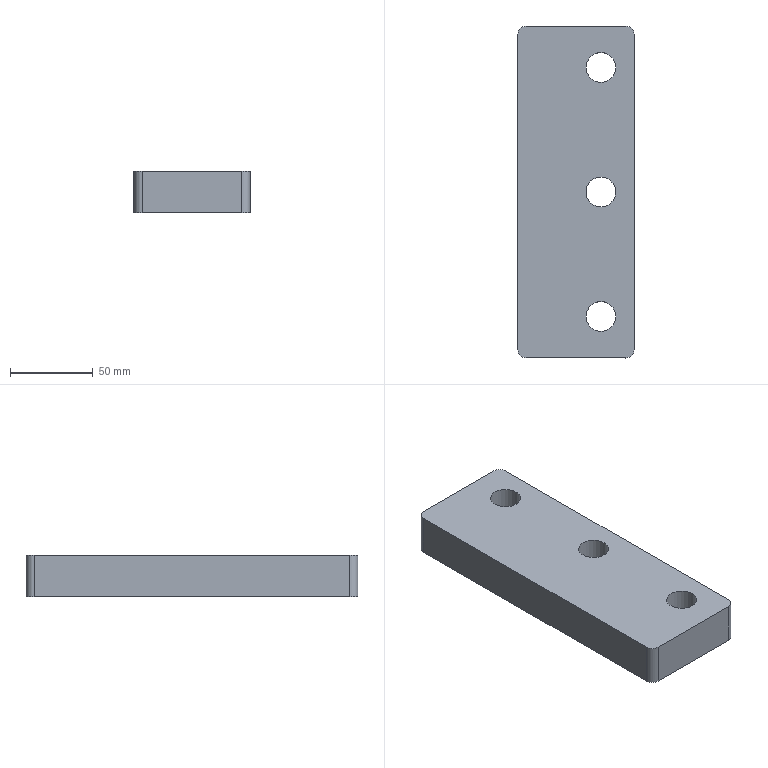Part | NX | features MAIN_BODY 2 | 1 solid | 13 faces | box 70 x 200 x 25 mm | volume 330378 mm3 | cylinder 7 | plane 6 | commonest cylinder face diameters 10 x4 18 x3
STEP:
#1=CARTESIAN_POINT('',(590.,740.,55.));
#2=VERTEX_POINT('',#1);
#3=CARTESIAN_POINT('',(650.,740.,55.));
#4=VERTEX_POINT('',#3);
#5=CARTESIAN_POINT('',(585.,740.,55.));
#6=DIRECTION('',(1.,0.,0.));
#7=VECTOR('',#6,1000.);
#8=LINE('',#5,#7);
#9=EDGE_CURVE('',#2,#4,#8,.T.);
#10=ORIENTED_EDGE('',*,*,#9,.T.);
#11=CARTESIAN_POINT('',(650.,740.,30.));
#12=VERTEX_POINT('',#11);
#13=CARTESIAN_POINT('',(650.,740.,30.));
#14=DIRECTION('',(0.,0.,1.));
#15=VECTOR('',#14,1000.);
#16=LINE('',#13,#15);
#17=EDGE_CURVE('',#12,#4,#16,.T.);
#18=ORIENTED_EDGE('',*,*,#17,.F.);
#19=CARTESIAN_POINT('',(590.,740.,30.));
#20=VERTEX_POINT('',#19);
#21=CARTESIAN_POINT('',(585.,740.,30.));
#22=DIRECTION('',(1.,0.,0.));
#23=VECTOR('',#22,1000.);
#24=LINE('',#21,#23);
#25=EDGE_CURVE('',#20,#12,#24,.T.);
#26=ORIENTED_EDGE('',*,*,#25,.F.);
#27=CARTESIAN_POINT('',(590.,740.,30.));
#28=DIRECTION('',(0.,0.,1.));
#29=VECTOR('',#28,1000.);
#30=LINE('',#27,#29);
#31=EDGE_CURVE('',#2,#20,#30,.F.);
#32=ORIENTED_EDGE('',*,*,#31,.F.);
#33=EDGE_LOOP('',(#10,#18,#26,#32));
#34=FACE_BOUND('',#33,.T.);
#35=CARTESIAN_POINT('',(585.,740.,30.));
#36=DIRECTION('',(0.,1.,0.));
#37=DIRECTION('',(-1.,0.,0.));
#38=AXIS2_PLACEMENT_3D('',#35,#36,#37);
#39=PLANE('',#38);
#40=ADVANCED_FACE('',(#34),#39,.T.);
#41=CARTESIAN_POINT('',(655.,735.,30.));
#42=VERTEX_POINT('',#41);
#43=CARTESIAN_POINT('',(655.,545.,30.));
#44=VERTEX_POINT('',#43);
#45=CARTESIAN_POINT('',(655.,740.,30.));
#46=DIRECTION('',(0.,-1.,0.));
#47=VECTOR('',#46,1000.);
#48=LINE('',#45,#47);
#49=EDGE_CURVE('',#42,#44,#48,.T.);
#50=ORIENTED_EDGE('',*,*,#49,.F.);
#51=CARTESIAN_POINT('',(655.,735.,55.));
#52=VERTEX_POINT('',#51);
#53=CARTESIAN_POINT('',(655.,735.,30.));
#54=DIRECTION('',(0.,0.,1.));
#55=VECTOR('',#54,1000.);
#56=LINE('',#53,#55);
#57=EDGE_CURVE('',#52,#42,#56,.F.);
#58=ORIENTED_EDGE('',*,*,#57,.F.);
#59=CARTESIAN_POINT('',(655.,545.,55.));
#60=VERTEX_POINT('',#59);
#61=CARTESIAN_POINT('',(655.,740.,55.));
#62=DIRECTION('',(0.,-1.,0.));
#63=VECTOR('',#62,1000.);
#64=LINE('',#61,#63);
#65=EDGE_CURVE('',#52,#60,#64,.T.);
#66=ORIENTED_EDGE('',*,*,#65,.T.);
#67=CARTESIAN_POINT('',(655.,545.,30.));
#68=DIRECTION('',(0.,0.,1.));
#69=VECTOR('',#68,1000.);
#70=LINE('',#67,#69);
#71=EDGE_CURVE('',#44,#60,#70,.T.);
#72=ORIENTED_EDGE('',*,*,#71,.F.);
#73=EDGE_LOOP('',(#50,#58,#66,#72));
#74=FACE_BOUND('',#73,.T.);
#75=CARTESIAN_POINT('',(655.,740.,30.));
#76=DIRECTION('',(1.,0.,0.));
#77=DIRECTION('',(0.,1.,0.));
#78=AXIS2_PLACEMENT_3D('',#75,#76,#77);
#79=PLANE('',#78);
#80=ADVANCED_FACE('',(#74),#79,.T.);
#81=CARTESIAN_POINT('',(650.,540.,30.));
#82=VERTEX_POINT('',#81);
#83=CARTESIAN_POINT('',(590.,540.,30.));
#84=VERTEX_POINT('',#83);
#85=CARTESIAN_POINT('',(655.,540.,30.));
#86=DIRECTION('',(-1.,0.,0.));
#87=VECTOR('',#86,1000.);
#88=LINE('',#85,#87);
#89=EDGE_CURVE('',#82,#84,#88,.T.);
#90=ORIENTED_EDGE('',*,*,#89,.F.);
#91=CARTESIAN_POINT('',(650.,540.,55.));
#92=VERTEX_POINT('',#91);
#93=CARTESIAN_POINT('',(650.,540.,30.));
#94=DIRECTION('',(0.,0.,1.));
#95=VECTOR('',#94,1000.);
#96=LINE('',#93,#95);
#97=EDGE_CURVE('',#92,#82,#96,.F.);
#98=ORIENTED_EDGE('',*,*,#97,.F.);
#99=CARTESIAN_POINT('',(590.,540.,55.));
#100=VERTEX_POINT('',#99);
#101=CARTESIAN_POINT('',(655.,540.,55.));
#102=DIRECTION('',(-1.,0.,0.));
#103=VECTOR('',#102,1000.);
#104=LINE('',#101,#103);
#105=EDGE_CURVE('',#92,#100,#104,.T.);
#106=ORIENTED_EDGE('',*,*,#105,.T.);
#107=CARTESIAN_POINT('',(590.,540.,30.));
#108=DIRECTION('',(0.,0.,1.));
#109=VECTOR('',#108,1000.);
#110=LINE('',#107,#109);
#111=EDGE_CURVE('',#84,#100,#110,.T.);
#112=ORIENTED_EDGE('',*,*,#111,.F.);
#113=EDGE_LOOP('',(#90,#98,#106,#112));
#114=FACE_BOUND('',#113,.T.);
#115=CARTESIAN_POINT('',(655.,540.,30.));
#116=DIRECTION('',(0.,-1.,0.));
#117=DIRECTION('',(0.,0.,-1.));
#118=AXIS2_PLACEMENT_3D('',#115,#116,#117);
#119=PLANE('',#118);
#120=ADVANCED_FACE('',(#114),#119,.T.);
#121=CARTESIAN_POINT('',(585.,545.,55.));
#122=VERTEX_POINT('',#121);
#123=CARTESIAN_POINT('',(585.,735.,55.));
#124=VERTEX_POINT('',#123);
#125=CARTESIAN_POINT('',(585.,540.,55.));
#126=DIRECTION('',(0.,1.,0.));
#127=VECTOR('',#126,1000.);
#128=LINE('',#125,#127);
#129=EDGE_CURVE('',#122,#124,#128,.T.);
#130=ORIENTED_EDGE('',*,*,#129,.T.);
#131=CARTESIAN_POINT('',(585.,735.,30.));
#132=VERTEX_POINT('',#131);
#133=CARTESIAN_POINT('',(585.,735.,30.));
#134=DIRECTION('',(0.,0.,1.));
#135=VECTOR('',#134,1000.);
#136=LINE('',#133,#135);
#137=EDGE_CURVE('',#132,#124,#136,.T.);
#138=ORIENTED_EDGE('',*,*,#137,.F.);
#139=CARTESIAN_POINT('',(585.,545.,30.));
#140=VERTEX_POINT('',#139);
#141=CARTESIAN_POINT('',(585.,540.,30.));
#142=DIRECTION('',(0.,1.,0.));
#143=VECTOR('',#142,1000.);
#144=LINE('',#141,#143);
#145=EDGE_CURVE('',#140,#132,#144,.T.);
#146=ORIENTED_EDGE('',*,*,#145,.F.);
#147=CARTESIAN_POINT('',(585.,545.,30.));
#148=DIRECTION('',(0.,0.,1.));
#149=VECTOR('',#148,1000.);
#150=LINE('',#147,#149);
#151=EDGE_CURVE('',#122,#140,#150,.F.);
#152=ORIENTED_EDGE('',*,*,#151,.F.);
#153=EDGE_LOOP('',(#130,#138,#146,#152));
#154=FACE_BOUND('',#153,.T.);
#155=CARTESIAN_POINT('',(585.,540.,30.));
#156=DIRECTION('',(-1.,0.,0.));
#157=DIRECTION('',(0.,0.,-1.));
#158=AXIS2_PLACEMENT_3D('',#155,#156,#157);
#159=PLANE('',#158);
#160=ADVANCED_FACE('',(#154),#159,.T.);
#161=CARTESIAN_POINT('',(635.,556.,30.));
#162=VERTEX_POINT('',#161);
#163=CARTESIAN_POINT('',(635.,565.,30.));
#164=DIRECTION('',(0.,0.,-1.));
#165=DIRECTION('',(0.,-1.,0.));
#166=AXIS2_PLACEMENT_3D('',#163,#164,#165);
#167=CIRCLE('',#166,9.);
#168=EDGE_CURVE('',#162,#162,#167,.T.);
#169=ORIENTED_EDGE('',*,*,#168,.F.);
#170=EDGE_LOOP('',(#169));
#171=FACE_BOUND('',#170,.T.);
#172=CARTESIAN_POINT('',(635.,631.,30.));
#173=VERTEX_POINT('',#172);
#174=CARTESIAN_POINT('',(635.,640.,30.));
#175=DIRECTION('',(0.,0.,-1.));
#176=DIRECTION('',(0.,-1.,0.));
#177=AXIS2_PLACEMENT_3D('',#174,#175,#176);
#178=CIRCLE('',#177,9.);
#179=EDGE_CURVE('',#173,#173,#178,.T.);
#180=ORIENTED_EDGE('',*,*,#179,.F.);
#181=EDGE_LOOP('',(#180));
#182=FACE_BOUND('',#181,.T.);
#183=CARTESIAN_POINT('',(635.,706.,30.));
#184=VERTEX_POINT('',#183);
#185=CARTESIAN_POINT('',(635.,715.,30.));
#186=DIRECTION('',(0.,0.,-1.));
#187=DIRECTION('',(0.,-1.,0.));
#188=AXIS2_PLACEMENT_3D('',#185,#186,#187);
#189=CIRCLE('',#188,9.);
#190=EDGE_CURVE('',#184,#184,#189,.T.);
#191=ORIENTED_EDGE('',*,*,#190,.F.);
#192=EDGE_LOOP('',(#191));
#193=FACE_BOUND('',#192,.T.);
#194=ORIENTED_EDGE('',*,*,#145,.T.);
#195=CARTESIAN_POINT('',(590.,735.,30.));
#196=DIRECTION('',(0.,0.,-1.));
#197=DIRECTION('',(0.,-1.,0.));
#198=AXIS2_PLACEMENT_3D('',#195,#196,#197);
#199=CIRCLE('',#198,5.);
#200=EDGE_CURVE('',#20,#132,#199,.F.);
#201=ORIENTED_EDGE('',*,*,#200,.F.);
#202=ORIENTED_EDGE('',*,*,#25,.T.);
#203=CARTESIAN_POINT('',(650.,735.,30.));
#204=DIRECTION('',(0.,0.,-1.));
#205=DIRECTION('',(0.,-1.,0.));
#206=AXIS2_PLACEMENT_3D('',#203,#204,#205);
#207=CIRCLE('',#206,5.);
#208=EDGE_CURVE('',#42,#12,#207,.F.);
#209=ORIENTED_EDGE('',*,*,#208,.F.);
#210=ORIENTED_EDGE('',*,*,#49,.T.);
#211=CARTESIAN_POINT('',(650.,545.,30.));
#212=DIRECTION('',(0.,0.,-1.));
#213=DIRECTION('',(0.,-1.,0.));
#214=AXIS2_PLACEMENT_3D('',#211,#212,#213);
#215=CIRCLE('',#214,5.);
#216=EDGE_CURVE('',#82,#44,#215,.F.);
#217=ORIENTED_EDGE('',*,*,#216,.F.);
#218=ORIENTED_EDGE('',*,*,#89,.T.);
#219=CARTESIAN_POINT('',(590.,545.,30.));
#220=DIRECTION('',(0.,0.,-1.));
#221=DIRECTION('',(0.,-1.,0.));
#222=AXIS2_PLACEMENT_3D('',#219,#220,#221);
#223=CIRCLE('',#222,5.);
#224=EDGE_CURVE('',#140,#84,#223,.F.);
#225=ORIENTED_EDGE('',*,*,#224,.F.);
#226=EDGE_LOOP('',(#194,#201,#202,#209,#210,#217,#218,#225));
#227=FACE_BOUND('',#226,.T.);
#228=CARTESIAN_POINT('',(655.,740.,30.));
#229=DIRECTION('',(0.,0.,1.));
#230=DIRECTION('',(0.,-1.,0.));
#231=AXIS2_PLACEMENT_3D('',#228,#229,#230);
#232=PLANE('',#231);
#233=ADVANCED_FACE('',(#171,#182,#193,#227),#232,.F.);
#234=CARTESIAN_POINT('',(635.,556.,55.));
#235=VERTEX_POINT('',#234);
#236=CARTESIAN_POINT('',(635.,565.,55.));
#237=DIRECTION('',(0.,0.,-1.));
#238=DIRECTION('',(0.,-1.,0.));
#239=AXIS2_PLACEMENT_3D('',#236,#237,#238);
#240=CIRCLE('',#239,9.);
#241=EDGE_CURVE('',#235,#235,#240,.T.);
#242=ORIENTED_EDGE('',*,*,#241,.T.);
#243=EDGE_LOOP('',(#242));
#244=FACE_BOUND('',#243,.T.);
#245=CARTESIAN_POINT('',(635.,631.,55.));
#246=VERTEX_POINT('',#245);
#247=CARTESIAN_POINT('',(635.,640.,55.));
#248=DIRECTION('',(0.,0.,-1.));
#249=DIRECTION('',(0.,-1.,0.));
#250=AXIS2_PLACEMENT_3D('',#247,#248,#249);
#251=CIRCLE('',#250,9.);
#252=EDGE_CURVE('',#246,#246,#251,.T.);
#253=ORIENTED_EDGE('',*,*,#252,.T.);
#254=EDGE_LOOP('',(#253));
#255=FACE_BOUND('',#254,.T.);
#256=CARTESIAN_POINT('',(635.,706.,55.));
#257=VERTEX_POINT('',#256);
#258=CARTESIAN_POINT('',(635.,715.,55.));
#259=DIRECTION('',(0.,0.,-1.));
#260=DIRECTION('',(0.,-1.,0.));
#261=AXIS2_PLACEMENT_3D('',#258,#259,#260);
#262=CIRCLE('',#261,9.);
#263=EDGE_CURVE('',#257,#257,#262,.T.);
#264=ORIENTED_EDGE('',*,*,#263,.T.);
#265=EDGE_LOOP('',(#264));
#266=FACE_BOUND('',#265,.T.);
#267=ORIENTED_EDGE('',*,*,#105,.F.);
#268=CARTESIAN_POINT('',(650.,545.,55.));
#269=DIRECTION('',(0.,0.,-1.));
#270=DIRECTION('',(0.,-1.,0.));
#271=AXIS2_PLACEMENT_3D('',#268,#269,#270);
#272=CIRCLE('',#271,5.);
#273=EDGE_CURVE('',#60,#92,#272,.T.);
#274=ORIENTED_EDGE('',*,*,#273,.F.);
#275=ORIENTED_EDGE('',*,*,#65,.F.);
#276=CARTESIAN_POINT('',(650.,735.,55.));
#277=DIRECTION('',(0.,0.,-1.));
#278=DIRECTION('',(0.,-1.,0.));
#279=AXIS2_PLACEMENT_3D('',#276,#277,#278);
#280=CIRCLE('',#279,5.);
#281=EDGE_CURVE('',#4,#52,#280,.T.);
#282=ORIENTED_EDGE('',*,*,#281,.F.);
#283=ORIENTED_EDGE('',*,*,#9,.F.);
#284=CARTESIAN_POINT('',(590.,735.,55.));
#285=DIRECTION('',(0.,0.,-1.));
#286=DIRECTION('',(0.,-1.,0.));
#287=AXIS2_PLACEMENT_3D('',#284,#285,#286);
#288=CIRCLE('',#287,5.);
#289=EDGE_CURVE('',#124,#2,#288,.T.);
#290=ORIENTED_EDGE('',*,*,#289,.F.);
#291=ORIENTED_EDGE('',*,*,#129,.F.);
#292=CARTESIAN_POINT('',(590.,545.,55.));
#293=DIRECTION('',(0.,0.,-1.));
#294=DIRECTION('',(0.,-1.,0.));
#295=AXIS2_PLACEMENT_3D('',#292,#293,#294);
#296=CIRCLE('',#295,5.);
#297=EDGE_CURVE('',#100,#122,#296,.T.);
#298=ORIENTED_EDGE('',*,*,#297,.F.);
#299=EDGE_LOOP('',(#267,#274,#275,#282,#283,#290,#291,#298));
#300=FACE_BOUND('',#299,.T.);
#301=CARTESIAN_POINT('',(655.,740.,55.));
#302=DIRECTION('',(0.,0.,1.));
#303=DIRECTION('',(0.,-1.,0.));
#304=AXIS2_PLACEMENT_3D('',#301,#302,#303);
#305=PLANE('',#304);
#306=ADVANCED_FACE('',(#244,#255,#266,#300),#305,.T.);
#307=ORIENTED_EDGE('',*,*,#263,.F.);
#308=EDGE_LOOP('',(#307));
#309=FACE_BOUND('',#308,.T.);
#310=ORIENTED_EDGE('',*,*,#190,.T.);
#311=EDGE_LOOP('',(#310));
#312=FACE_BOUND('',#311,.T.);
#313=CARTESIAN_POINT('',(635.,715.,30.));
#314=DIRECTION('',(0.,0.,1.));
#315=DIRECTION('',(0.,-1.,0.));
#316=AXIS2_PLACEMENT_3D('',#313,#314,#315);
#317=CYLINDRICAL_SURFACE('',#316,9.);
#318=ADVANCED_FACE('',(#309,#312),#317,.F.);
#319=ORIENTED_EDGE('',*,*,#252,.F.);
#320=EDGE_LOOP('',(#319));
#321=FACE_BOUND('',#320,.T.);
#322=ORIENTED_EDGE('',*,*,#179,.T.);
#323=EDGE_LOOP('',(#322));
#324=FACE_BOUND('',#323,.T.);
#325=CARTESIAN_POINT('',(635.,640.,30.));
#326=DIRECTION('',(0.,0.,1.));
#327=DIRECTION('',(0.,-1.,0.));
#328=AXIS2_PLACEMENT_3D('',#325,#326,#327);
#329=CYLINDRICAL_SURFACE('',#328,9.);
#330=ADVANCED_FACE('',(#321,#324),#329,.F.);
#331=ORIENTED_EDGE('',*,*,#241,.F.);
#332=EDGE_LOOP('',(#331));
#333=FACE_BOUND('',#332,.T.);
#334=ORIENTED_EDGE('',*,*,#168,.T.);
#335=EDGE_LOOP('',(#334));
#336=FACE_BOUND('',#335,.T.);
#337=CARTESIAN_POINT('',(635.,565.,30.));
#338=DIRECTION('',(0.,0.,1.));
#339=DIRECTION('',(0.,-1.,0.));
#340=AXIS2_PLACEMENT_3D('',#337,#338,#339);
#341=CYLINDRICAL_SURFACE('',#340,9.);
#342=ADVANCED_FACE('',(#333,#336),#341,.F.);
#343=ORIENTED_EDGE('',*,*,#224,.T.);
#344=ORIENTED_EDGE('',*,*,#111,.T.);
#345=ORIENTED_EDGE('',*,*,#297,.T.);
#346=ORIENTED_EDGE('',*,*,#151,.T.);
#347=EDGE_LOOP('',(#343,#344,#345,#346));
#348=FACE_BOUND('',#347,.T.);
#349=CARTESIAN_POINT('',(590.,545.,30.));
#350=DIRECTION('',(0.,0.,1.));
#351=DIRECTION('',(0.,-1.,0.));
#352=AXIS2_PLACEMENT_3D('',#349,#350,#351);
#353=CYLINDRICAL_SURFACE('',#352,5.);
#354=ADVANCED_FACE('',(#348),#353,.T.);
#355=ORIENTED_EDGE('',*,*,#216,.T.);
#356=ORIENTED_EDGE('',*,*,#71,.T.);
#357=ORIENTED_EDGE('',*,*,#273,.T.);
#358=ORIENTED_EDGE('',*,*,#97,.T.);
#359=EDGE_LOOP('',(#355,#356,#357,#358));
#360=FACE_BOUND('',#359,.T.);
#361=CARTESIAN_POINT('',(650.,545.,30.));
#362=DIRECTION('',(0.,0.,1.));
#363=DIRECTION('',(0.,-1.,0.));
#364=AXIS2_PLACEMENT_3D('',#361,#362,#363);
#365=CYLINDRICAL_SURFACE('',#364,5.);
#366=ADVANCED_FACE('',(#360),#365,.T.);
#367=ORIENTED_EDGE('',*,*,#200,.T.);
#368=ORIENTED_EDGE('',*,*,#137,.T.);
#369=ORIENTED_EDGE('',*,*,#289,.T.);
#370=ORIENTED_EDGE('',*,*,#31,.T.);
#371=EDGE_LOOP('',(#367,#368,#369,#370));
#372=FACE_BOUND('',#371,.T.);
#373=CARTESIAN_POINT('',(590.,735.,30.));
#374=DIRECTION('',(0.,0.,1.));
#375=DIRECTION('',(0.,-1.,0.));
#376=AXIS2_PLACEMENT_3D('',#373,#374,#375);
#377=CYLINDRICAL_SURFACE('',#376,5.);
#378=ADVANCED_FACE('',(#372),#377,.T.);
#379=ORIENTED_EDGE('',*,*,#208,.T.);
#380=ORIENTED_EDGE('',*,*,#17,.T.);
#381=ORIENTED_EDGE('',*,*,#281,.T.);
#382=ORIENTED_EDGE('',*,*,#57,.T.);
#383=EDGE_LOOP('',(#379,#380,#381,#382));
#384=FACE_BOUND('',#383,.T.);
#385=CARTESIAN_POINT('',(650.,735.,30.));
#386=DIRECTION('',(0.,0.,1.));
#387=DIRECTION('',(0.,-1.,0.));
#388=AXIS2_PLACEMENT_3D('',#385,#386,#387);
#389=CYLINDRICAL_SURFACE('',#388,5.);
#390=ADVANCED_FACE('',(#384),#389,.T.);
#391=CLOSED_SHELL('',(#40,#80,#120,#160,#233,#306,#318,#330,#342,#354,#366,#378,#390));
#392=MANIFOLD_SOLID_BREP('',#391);
#393=(LENGTH_UNIT()NAMED_UNIT(*)SI_UNIT(.MILLI.,.METRE.));
#394=UNCERTAINTY_MEASURE_WITH_UNIT(LENGTH_MEASURE(0.00001),#393,'','');
#395=(NAMED_UNIT(*)PLANE_ANGLE_UNIT()SI_UNIT($,.RADIAN.));
#396=(NAMED_UNIT(*)SI_UNIT($,.STERADIAN.)SOLID_ANGLE_UNIT());
#397=(GEOMETRIC_REPRESENTATION_CONTEXT(3)GLOBAL_UNCERTAINTY_ASSIGNED_CONTEXT((#394))GLOBAL_UNIT_ASSIGNED_CONTEXT((#393,#395,#396))REPRESENTATION_CONTEXT('',''));
#398=ADVANCED_BREP_SHAPE_REPRESENTATION('',(#392),#397);